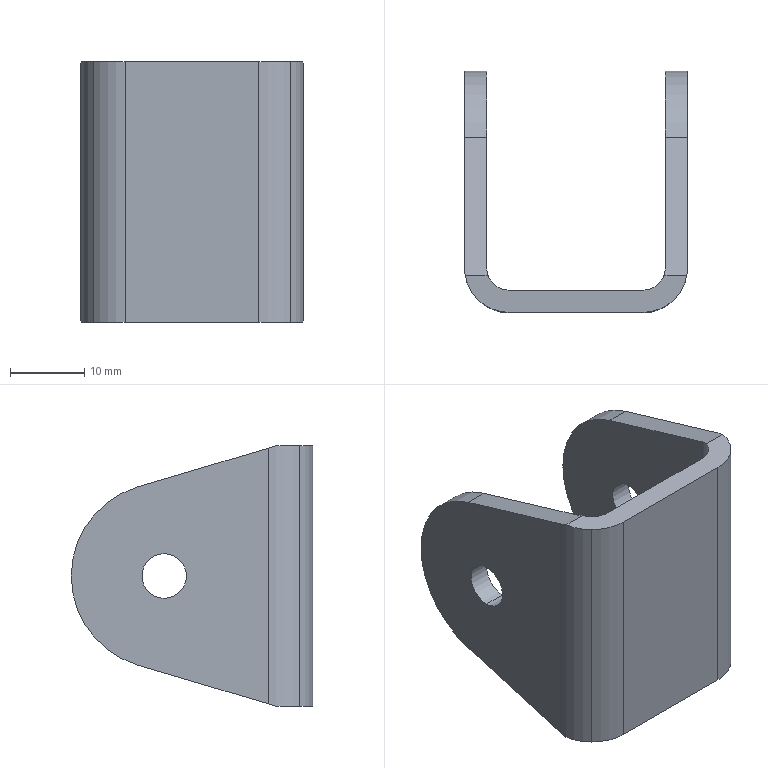Part | SolidWorks | features BaseBody 1 | 1 solid | 26 faces | box 30 x 32.5 x 35 mm | volume 7224 mm3 | cylinder 14 | plane 12 | commonest cylinder face diameters 6 x8 12 x4 25 x2
STEP:
#1=CARTESIAN_POINT('',(6.626,51.912,-683.821));
#2=VERTEX_POINT('',#1);
#3=CARTESIAN_POINT('',(6.626,51.912,-689.821));
#4=VERTEX_POINT('',#3);
#5=CARTESIAN_POINT('',(6.626,51.912,-686.821));
#6=DIRECTION('',(1.,0.,0.));
#7=DIRECTION('',(0.,0.,-1.));
#8=AXIS2_PLACEMENT_3D('',#5,#6,#7);
#9=CIRCLE('',#8,3.);
#10=EDGE_CURVE('',#2,#4,#9,.T.);
#11=ORIENTED_EDGE('',*,*,#10,.F.);
#12=CARTESIAN_POINT('',(9.626,51.912,-683.821));
#13=VERTEX_POINT('',#12);
#14=CARTESIAN_POINT('',(20.626,51.912,-683.821));
#15=DIRECTION('',(1.,0.,0.));
#16=VECTOR('',#15,1000.);
#17=LINE('',#14,#16);
#18=EDGE_CURVE('',#2,#13,#17,.T.);
#19=ORIENTED_EDGE('',*,*,#18,.T.);
#20=CARTESIAN_POINT('',(9.626,51.912,-689.821));
#21=VERTEX_POINT('',#20);
#22=CARTESIAN_POINT('',(9.626,51.912,-686.821));
#23=DIRECTION('',(-1.,0.,0.));
#24=DIRECTION('',(0.,0.,-1.));
#25=AXIS2_PLACEMENT_3D('',#22,#23,#24);
#26=CIRCLE('',#25,3.);
#27=EDGE_CURVE('',#21,#13,#26,.T.);
#28=ORIENTED_EDGE('',*,*,#27,.F.);
#29=CARTESIAN_POINT('',(20.626,51.912,-689.821));
#30=DIRECTION('',(1.,0.,0.));
#31=VECTOR('',#30,1000.);
#32=LINE('',#29,#31);
#33=EDGE_CURVE('',#4,#21,#32,.T.);
#34=ORIENTED_EDGE('',*,*,#33,.F.);
#35=EDGE_LOOP('',(#11,#19,#28,#34));
#36=FACE_OUTER_BOUND('',#35,.T.);
#37=CARTESIAN_POINT('',(20.626,51.912,-686.821));
#38=DIRECTION('',(1.,0.,0.));
#39=DIRECTION('',(0.,0.,-1.));
#40=AXIS2_PLACEMENT_3D('',#37,#38,#39);
#41=CYLINDRICAL_SURFACE('',#40,3.);
#42=ADVANCED_FACE('',(#36),#41,.F.);
#43=CARTESIAN_POINT('',(33.626,51.912,-683.821));
#44=VERTEX_POINT('',#43);
#45=CARTESIAN_POINT('',(33.626,51.912,-689.821));
#46=VERTEX_POINT('',#45);
#47=CARTESIAN_POINT('',(33.626,51.912,-686.821));
#48=DIRECTION('',(1.,0.,0.));
#49=DIRECTION('',(0.,0.,-1.));
#50=AXIS2_PLACEMENT_3D('',#47,#48,#49);
#51=CIRCLE('',#50,3.);
#52=EDGE_CURVE('',#44,#46,#51,.T.);
#53=ORIENTED_EDGE('',*,*,#52,.F.);
#54=CARTESIAN_POINT('',(36.626,51.912,-683.821));
#55=VERTEX_POINT('',#54);
#56=CARTESIAN_POINT('',(20.626,51.912,-683.821));
#57=DIRECTION('',(1.,0.,0.));
#58=VECTOR('',#57,1000.);
#59=LINE('',#56,#58);
#60=EDGE_CURVE('',#44,#55,#59,.T.);
#61=ORIENTED_EDGE('',*,*,#60,.T.);
#62=CARTESIAN_POINT('',(36.626,51.912,-689.821));
#63=VERTEX_POINT('',#62);
#64=CARTESIAN_POINT('',(36.626,51.912,-686.821));
#65=DIRECTION('',(-1.,0.,0.));
#66=DIRECTION('',(0.,0.,-1.));
#67=AXIS2_PLACEMENT_3D('',#64,#65,#66);
#68=CIRCLE('',#67,3.);
#69=EDGE_CURVE('',#63,#55,#68,.T.);
#70=ORIENTED_EDGE('',*,*,#69,.F.);
#71=CARTESIAN_POINT('',(20.626,51.912,-689.821));
#72=DIRECTION('',(1.,0.,0.));
#73=VECTOR('',#72,1000.);
#74=LINE('',#71,#73);
#75=EDGE_CURVE('',#46,#63,#74,.T.);
#76=ORIENTED_EDGE('',*,*,#75,.F.);
#77=EDGE_LOOP('',(#53,#61,#70,#76));
#78=FACE_OUTER_BOUND('',#77,.T.);
#79=CARTESIAN_POINT('',(20.626,51.912,-686.821));
#80=DIRECTION('',(1.,0.,0.));
#81=DIRECTION('',(0.,0.,-1.));
#82=AXIS2_PLACEMENT_3D('',#79,#80,#81);
#83=CYLINDRICAL_SURFACE('',#82,3.);
#84=ADVANCED_FACE('',(#78),#83,.F.);
#85=CARTESIAN_POINT('',(30.626,31.912,-704.321));
#86=VERTEX_POINT('',#85);
#87=CARTESIAN_POINT('',(34.868,33.67,-704.321));
#88=VERTEX_POINT('',#87);
#89=CARTESIAN_POINT('',(30.626,37.912,-704.321));
#90=DIRECTION('',(0.,0.,1.));
#91=DIRECTION('',(0.7071,-0.7071,0.));
#92=AXIS2_PLACEMENT_3D('',#89,#90,#91);
#93=CIRCLE('',#92,6.);
#94=EDGE_CURVE('',#86,#88,#93,.T.);
#95=ORIENTED_EDGE('',*,*,#94,.T.);
#96=CARTESIAN_POINT('',(34.868,33.67,-669.321));
#97=VERTEX_POINT('',#96);
#98=CARTESIAN_POINT('',(34.868,33.67,-695.571));
#99=DIRECTION('',(0.,0.,1.));
#100=VECTOR('',#99,1000.);
#101=LINE('',#98,#100);
#102=EDGE_CURVE('',#88,#97,#101,.T.);
#103=ORIENTED_EDGE('',*,*,#102,.T.);
#104=CARTESIAN_POINT('',(30.626,31.912,-669.321));
#105=VERTEX_POINT('',#104);
#106=CARTESIAN_POINT('',(30.626,37.912,-669.321));
#107=DIRECTION('',(0.,0.,-1.));
#108=DIRECTION('',(0.7071,-0.7071,0.));
#109=AXIS2_PLACEMENT_3D('',#106,#107,#108);
#110=CIRCLE('',#109,6.);
#111=EDGE_CURVE('',#97,#105,#110,.T.);
#112=ORIENTED_EDGE('',*,*,#111,.T.);
#113=CARTESIAN_POINT('',(30.626,31.912,-695.571));
#114=DIRECTION('',(0.,0.,-1.));
#115=VECTOR('',#114,1000.);
#116=LINE('',#113,#115);
#117=EDGE_CURVE('',#105,#86,#116,.T.);
#118=ORIENTED_EDGE('',*,*,#117,.T.);
#119=EDGE_LOOP('',(#95,#103,#112,#118));
#120=FACE_OUTER_BOUND('',#119,.T.);
#121=CARTESIAN_POINT('',(30.626,37.912,-695.571));
#122=DIRECTION('',(0.,0.,1.));
#123=DIRECTION('',(0.7071,-0.7071,0.));
#124=AXIS2_PLACEMENT_3D('',#121,#122,#123);
#125=CYLINDRICAL_SURFACE('',#124,6.);
#126=ADVANCED_FACE('',(#120),#125,.T.);
#127=CARTESIAN_POINT('',(6.71,36.912,-704.321));
#128=VERTEX_POINT('',#127);
#129=CARTESIAN_POINT('',(8.383,33.67,-704.321));
#130=VERTEX_POINT('',#129);
#131=CARTESIAN_POINT('',(12.626,37.912,-704.321));
#132=DIRECTION('',(0.,0.,1.));
#133=DIRECTION('',(-0.7071,-0.7071,0.));
#134=AXIS2_PLACEMENT_3D('',#131,#132,#133);
#135=CIRCLE('',#134,6.);
#136=EDGE_CURVE('',#128,#130,#135,.T.);
#137=ORIENTED_EDGE('',*,*,#136,.T.);
#138=CARTESIAN_POINT('',(8.383,33.67,-669.321));
#139=VERTEX_POINT('',#138);
#140=CARTESIAN_POINT('',(8.383,33.67,-695.571));
#141=DIRECTION('',(0.,0.,1.));
#142=VECTOR('',#141,1000.);
#143=LINE('',#140,#142);
#144=EDGE_CURVE('',#130,#139,#143,.T.);
#145=ORIENTED_EDGE('',*,*,#144,.T.);
#146=CARTESIAN_POINT('',(6.71,36.912,-669.321));
#147=VERTEX_POINT('',#146);
#148=CARTESIAN_POINT('',(12.626,37.912,-669.321));
#149=DIRECTION('',(0.,0.,-1.));
#150=DIRECTION('',(-0.7071,-0.7071,0.));
#151=AXIS2_PLACEMENT_3D('',#148,#149,#150);
#152=CIRCLE('',#151,6.);
#153=EDGE_CURVE('',#139,#147,#152,.T.);
#154=ORIENTED_EDGE('',*,*,#153,.T.);
#155=CARTESIAN_POINT('',(6.626,37.912,-669.619));
#156=VERTEX_POINT('',#155);
#157=CARTESIAN_POINT('',(6.71,36.912,-669.321));
#158=CARTESIAN_POINT('',(6.654,37.243,-669.42));
#159=CARTESIAN_POINT('',(6.626,37.577,-669.519));
#160=CARTESIAN_POINT('',(6.626,37.912,-669.619));
#161=(BOUNDED_CURVE()B_SPLINE_CURVE(3,(#157,#158,#159,#160),.UNSPECIFIED.,.F.,.T.)B_SPLINE_CURVE_WITH_KNOTS((4,4),(1.403,1.571),.UNSPECIFIED.)CURVE()GEOMETRIC_REPRESENTATION_ITEM()RATIONAL_B_SPLINE_CURVE((1.,0.9977,0.9977,1.))REPRESENTATION_ITEM(''));
#162=EDGE_CURVE('',#147,#156,#161,.T.);
#163=ORIENTED_EDGE('',*,*,#162,.T.);
#164=CARTESIAN_POINT('',(6.626,37.912,-704.024));
#165=VERTEX_POINT('',#164);
#166=CARTESIAN_POINT('',(6.626,37.912,-695.571));
#167=DIRECTION('',(0.,0.,-1.));
#168=VECTOR('',#167,1000.);
#169=LINE('',#166,#168);
#170=EDGE_CURVE('',#156,#165,#169,.T.);
#171=ORIENTED_EDGE('',*,*,#170,.T.);
#172=CARTESIAN_POINT('',(6.626,37.912,-704.024));
#173=CARTESIAN_POINT('',(6.626,37.577,-704.124));
#174=CARTESIAN_POINT('',(6.654,37.243,-704.223));
#175=CARTESIAN_POINT('',(6.71,36.912,-704.321));
#176=(BOUNDED_CURVE()B_SPLINE_CURVE(3,(#172,#173,#174,#175),.UNSPECIFIED.,.F.,.F.)B_SPLINE_CURVE_WITH_KNOTS((4,4),(4.712,4.88),.UNSPECIFIED.)CURVE()GEOMETRIC_REPRESENTATION_ITEM()RATIONAL_B_SPLINE_CURVE((1.,0.9977,0.9977,1.))REPRESENTATION_ITEM(''));
#177=EDGE_CURVE('',#165,#128,#176,.T.);
#178=ORIENTED_EDGE('',*,*,#177,.T.);
#179=EDGE_LOOP('',(#137,#145,#154,#163,#171,#178));
#180=FACE_OUTER_BOUND('',#179,.T.);
#181=CARTESIAN_POINT('',(12.626,37.912,-695.571));
#182=DIRECTION('',(0.,0.,1.));
#183=DIRECTION('',(-0.7071,-0.7071,0.));
#184=AXIS2_PLACEMENT_3D('',#181,#182,#183);
#185=CYLINDRICAL_SURFACE('',#184,6.);
#186=ADVANCED_FACE('',(#180),#185,.T.);
#187=CARTESIAN_POINT('',(30.626,34.912,-669.321));
#188=VERTEX_POINT('',#187);
#189=CARTESIAN_POINT('',(32.747,35.791,-669.321));
#190=VERTEX_POINT('',#189);
#191=CARTESIAN_POINT('',(30.626,37.912,-669.321));
#192=DIRECTION('',(0.,0.,1.));
#193=DIRECTION('',(0.7071,-0.7071,0.));
#194=AXIS2_PLACEMENT_3D('',#191,#192,#193);
#195=CIRCLE('',#194,3.);
#196=EDGE_CURVE('',#188,#190,#195,.T.);
#197=ORIENTED_EDGE('',*,*,#196,.T.);
#198=CARTESIAN_POINT('',(32.747,35.791,-704.321));
#199=VERTEX_POINT('',#198);
#200=CARTESIAN_POINT('',(32.747,35.791,-669.321));
#201=DIRECTION('',(0.,0.,-1.));
#202=VECTOR('',#201,1000.);
#203=LINE('',#200,#202);
#204=EDGE_CURVE('',#190,#199,#203,.T.);
#205=ORIENTED_EDGE('',*,*,#204,.T.);
#206=CARTESIAN_POINT('',(30.626,34.912,-704.321));
#207=VERTEX_POINT('',#206);
#208=CARTESIAN_POINT('',(30.626,37.912,-704.321));
#209=DIRECTION('',(0.,0.,1.));
#210=DIRECTION('',(0.7071,-0.7071,0.));
#211=AXIS2_PLACEMENT_3D('',#208,#209,#210);
#212=CIRCLE('',#211,3.);
#213=EDGE_CURVE('',#207,#199,#212,.T.);
#214=ORIENTED_EDGE('',*,*,#213,.F.);
#215=CARTESIAN_POINT('',(30.626,34.912,-669.321));
#216=DIRECTION('',(0.,0.,1.));
#217=VECTOR('',#216,1000.);
#218=LINE('',#215,#217);
#219=EDGE_CURVE('',#207,#188,#218,.T.);
#220=ORIENTED_EDGE('',*,*,#219,.T.);
#221=EDGE_LOOP('',(#197,#205,#214,#220));
#222=FACE_OUTER_BOUND('',#221,.T.);
#223=CARTESIAN_POINT('',(30.626,37.912,-669.321));
#224=DIRECTION('',(0.,0.,-1.));
#225=DIRECTION('',(0.7071,-0.7071,0.));
#226=AXIS2_PLACEMENT_3D('',#223,#224,#225);
#227=CYLINDRICAL_SURFACE('',#226,3.);
#228=ADVANCED_FACE('',(#222),#227,.F.);
#229=CARTESIAN_POINT('',(10.504,35.791,-669.321));
#230=VERTEX_POINT('',#229);
#231=CARTESIAN_POINT('',(9.797,36.912,-669.321));
#232=VERTEX_POINT('',#231);
#233=CARTESIAN_POINT('',(12.626,37.912,-669.321));
#234=DIRECTION('',(0.,0.,-1.));
#235=DIRECTION('',(-0.7071,-0.7071,0.));
#236=AXIS2_PLACEMENT_3D('',#233,#234,#235);
#237=CIRCLE('',#236,3.);
#238=EDGE_CURVE('',#230,#232,#237,.T.);
#239=ORIENTED_EDGE('',*,*,#238,.F.);
#240=CARTESIAN_POINT('',(10.504,35.791,-704.321));
#241=VERTEX_POINT('',#240);
#242=CARTESIAN_POINT('',(10.504,35.791,-669.321));
#243=DIRECTION('',(0.,0.,-1.));
#244=VECTOR('',#243,1000.);
#245=LINE('',#242,#244);
#246=EDGE_CURVE('',#230,#241,#245,.T.);
#247=ORIENTED_EDGE('',*,*,#246,.T.);
#248=CARTESIAN_POINT('',(9.797,36.912,-704.321));
#249=VERTEX_POINT('',#248);
#250=CARTESIAN_POINT('',(12.626,37.912,-704.321));
#251=DIRECTION('',(0.,0.,-1.));
#252=DIRECTION('',(-0.7071,-0.7071,0.));
#253=AXIS2_PLACEMENT_3D('',#250,#251,#252);
#254=CIRCLE('',#253,3.);
#255=EDGE_CURVE('',#241,#249,#254,.T.);
#256=ORIENTED_EDGE('',*,*,#255,.T.);
#257=CARTESIAN_POINT('',(9.626,37.912,-704.024));
#258=VERTEX_POINT('',#257);
#259=CARTESIAN_POINT('',(9.626,37.912,-704.024));
#260=CARTESIAN_POINT('',(9.626,37.571,-704.126));
#261=CARTESIAN_POINT('',(9.683,37.234,-704.226));
#262=CARTESIAN_POINT('',(9.797,36.912,-704.321));
#263=(BOUNDED_CURVE()B_SPLINE_CURVE(3,(#259,#260,#261,#262),.UNSPECIFIED.,.F.,.F.)B_SPLINE_CURVE_WITH_KNOTS((4,4),(4.712,5.052),.UNSPECIFIED.)CURVE()GEOMETRIC_REPRESENTATION_ITEM()RATIONAL_B_SPLINE_CURVE((1.,0.9904,0.9904,1.))REPRESENTATION_ITEM(''));
#264=EDGE_CURVE('',#258,#249,#263,.T.);
#265=ORIENTED_EDGE('',*,*,#264,.F.);
#266=CARTESIAN_POINT('',(9.626,37.912,-669.619));
#267=VERTEX_POINT('',#266);
#268=CARTESIAN_POINT('',(9.626,37.912,-669.321));
#269=DIRECTION('',(0.,0.,1.));
#270=VECTOR('',#269,1000.);
#271=LINE('',#268,#270);
#272=EDGE_CURVE('',#258,#267,#271,.T.);
#273=ORIENTED_EDGE('',*,*,#272,.T.);
#274=CARTESIAN_POINT('',(9.626,37.912,-669.619));
#275=CARTESIAN_POINT('',(9.626,37.571,-669.517));
#276=CARTESIAN_POINT('',(9.683,37.234,-669.417));
#277=CARTESIAN_POINT('',(9.797,36.912,-669.321));
#278=(BOUNDED_CURVE()B_SPLINE_CURVE(3,(#274,#275,#276,#277),.UNSPECIFIED.,.F.,.F.)B_SPLINE_CURVE_WITH_KNOTS((4,4),(4.712,5.052),.UNSPECIFIED.)CURVE()GEOMETRIC_REPRESENTATION_ITEM()RATIONAL_B_SPLINE_CURVE((1.,0.9904,0.9904,1.))REPRESENTATION_ITEM(''));
#279=EDGE_CURVE('',#267,#232,#278,.T.);
#280=ORIENTED_EDGE('',*,*,#279,.T.);
#281=EDGE_LOOP('',(#239,#247,#256,#265,#273,#280));
#282=FACE_OUTER_BOUND('',#281,.T.);
#283=CARTESIAN_POINT('',(12.626,37.912,-669.321));
#284=DIRECTION('',(0.,0.,-1.));
#285=DIRECTION('',(-0.7071,-0.7071,0.));
#286=AXIS2_PLACEMENT_3D('',#283,#284,#285);
#287=CYLINDRICAL_SURFACE('',#286,3.);
#288=ADVANCED_FACE('',(#282),#287,.F.);
#289=ORIENTED_EDGE('',*,*,#69,.T.);
#290=CARTESIAN_POINT('',(36.626,51.912,-686.821));
#291=DIRECTION('',(-1.,0.,0.));
#292=DIRECTION('',(0.,0.,-1.));
#293=AXIS2_PLACEMENT_3D('',#290,#291,#292);
#294=CIRCLE('',#293,3.);
#295=EDGE_CURVE('',#55,#63,#294,.T.);
#296=ORIENTED_EDGE('',*,*,#295,.T.);
#297=EDGE_LOOP('',(#289,#296));
#298=FACE_BOUND('',#297,.T.);
#299=CARTESIAN_POINT('',(36.626,37.912,-704.024));
#300=VERTEX_POINT('',#299);
#301=CARTESIAN_POINT('',(36.626,37.912,-669.619));
#302=VERTEX_POINT('',#301);
#303=CARTESIAN_POINT('',(36.626,37.912,-695.571));
#304=DIRECTION('',(0.,0.,1.));
#305=VECTOR('',#304,1000.);
#306=LINE('',#303,#305);
#307=EDGE_CURVE('',#300,#302,#306,.T.);
#308=ORIENTED_EDGE('',*,*,#307,.F.);
#309=CARTESIAN_POINT('',(36.626,55.474,-698.803));
#310=VERTEX_POINT('',#309);
#311=CARTESIAN_POINT('',(36.626,55.474,-698.803));
#312=DIRECTION('',(0.,-0.9585,-0.285));
#313=VECTOR('',#312,1000.);
#314=LINE('',#311,#313);
#315=EDGE_CURVE('',#310,#300,#314,.T.);
#316=ORIENTED_EDGE('',*,*,#315,.F.);
#317=CARTESIAN_POINT('',(36.626,55.474,-674.84));
#318=VERTEX_POINT('',#317);
#319=CARTESIAN_POINT('',(36.626,51.912,-686.821));
#320=DIRECTION('',(-1.,0.,0.));
#321=DIRECTION('',(0.,0.285,0.9585));
#322=AXIS2_PLACEMENT_3D('',#319,#320,#321);
#323=CIRCLE('',#322,12.5);
#324=EDGE_CURVE('',#318,#310,#323,.T.);
#325=ORIENTED_EDGE('',*,*,#324,.F.);
#326=CARTESIAN_POINT('',(36.626,36.912,-669.321));
#327=DIRECTION('',(0.,0.9585,-0.285));
#328=VECTOR('',#327,1000.);
#329=LINE('',#326,#328);
#330=EDGE_CURVE('',#302,#318,#329,.T.);
#331=ORIENTED_EDGE('',*,*,#330,.F.);
#332=EDGE_LOOP('',(#308,#316,#325,#331));
#333=FACE_OUTER_BOUND('',#332,.T.);
#334=CARTESIAN_POINT('',(36.626,43.822,-686.821));
#335=DIRECTION('',(-1.,0.,0.));
#336=DIRECTION('',(0.,0.,1.));
#337=AXIS2_PLACEMENT_3D('',#334,#335,#336);
#338=PLANE('',#337);
#339=ADVANCED_FACE('',(#298,#333),#338,.F.);
#340=CARTESIAN_POINT('',(6.626,51.912,-686.821));
#341=DIRECTION('',(1.,0.,0.));
#342=DIRECTION('',(0.,0.,-1.));
#343=AXIS2_PLACEMENT_3D('',#340,#341,#342);
#344=CIRCLE('',#343,3.);
#345=EDGE_CURVE('',#4,#2,#344,.T.);
#346=ORIENTED_EDGE('',*,*,#345,.T.);
#347=ORIENTED_EDGE('',*,*,#10,.T.);
#348=EDGE_LOOP('',(#346,#347));
#349=FACE_BOUND('',#348,.T.);
#350=ORIENTED_EDGE('',*,*,#170,.F.);
#351=CARTESIAN_POINT('',(6.626,55.474,-674.84));
#352=VERTEX_POINT('',#351);
#353=CARTESIAN_POINT('',(6.626,36.912,-669.321));
#354=DIRECTION('',(0.,0.9585,-0.285));
#355=VECTOR('',#354,1000.);
#356=LINE('',#353,#355);
#357=EDGE_CURVE('',#156,#352,#356,.T.);
#358=ORIENTED_EDGE('',*,*,#357,.T.);
#359=CARTESIAN_POINT('',(6.626,55.474,-698.803));
#360=VERTEX_POINT('',#359);
#361=CARTESIAN_POINT('',(6.626,51.912,-686.821));
#362=DIRECTION('',(-1.,0.,0.));
#363=DIRECTION('',(0.,0.285,0.9585));
#364=AXIS2_PLACEMENT_3D('',#361,#362,#363);
#365=CIRCLE('',#364,12.5);
#366=EDGE_CURVE('',#352,#360,#365,.T.);
#367=ORIENTED_EDGE('',*,*,#366,.T.);
#368=CARTESIAN_POINT('',(6.626,55.474,-698.803));
#369=DIRECTION('',(0.,-0.9585,-0.285));
#370=VECTOR('',#369,1000.);
#371=LINE('',#368,#370);
#372=EDGE_CURVE('',#360,#165,#371,.T.);
#373=ORIENTED_EDGE('',*,*,#372,.T.);
#374=EDGE_LOOP('',(#350,#358,#367,#373));
#375=FACE_OUTER_BOUND('',#374,.T.);
#376=CARTESIAN_POINT('',(6.626,43.822,-686.821));
#377=DIRECTION('',(-1.,0.,0.));
#378=DIRECTION('',(0.,0.,1.));
#379=AXIS2_PLACEMENT_3D('',#376,#377,#378);
#380=PLANE('',#379);
#381=ADVANCED_FACE('',(#349,#375),#380,.T.);
#382=CARTESIAN_POINT('',(33.626,55.474,-698.803));
#383=VERTEX_POINT('',#382);
#384=CARTESIAN_POINT('',(33.626,55.474,-674.84));
#385=VERTEX_POINT('',#384);
#386=CARTESIAN_POINT('',(33.626,51.912,-686.821));
#387=DIRECTION('',(1.,0.,0.));
#388=DIRECTION('',(0.,0.285,0.9585));
#389=AXIS2_PLACEMENT_3D('',#386,#387,#388);
#390=CIRCLE('',#389,12.5);
#391=EDGE_CURVE('',#383,#385,#390,.T.);
#392=ORIENTED_EDGE('',*,*,#391,.T.);
#393=CARTESIAN_POINT('',(36.626,55.474,-674.84));
#394=DIRECTION('',(-1.,0.,0.));
#395=VECTOR('',#394,1000.);
#396=LINE('',#393,#395);
#397=EDGE_CURVE('',#318,#385,#396,.T.);
#398=ORIENTED_EDGE('',*,*,#397,.F.);
#399=ORIENTED_EDGE('',*,*,#324,.T.);
#400=CARTESIAN_POINT('',(36.626,55.474,-698.803));
#401=DIRECTION('',(-1.,0.,0.));
#402=VECTOR('',#401,1000.);
#403=LINE('',#400,#402);
#404=EDGE_CURVE('',#310,#383,#403,.T.);
#405=ORIENTED_EDGE('',*,*,#404,.T.);
#406=EDGE_LOOP('',(#392,#398,#399,#405));
#407=FACE_OUTER_BOUND('',#406,.T.);
#408=CARTESIAN_POINT('',(36.626,51.912,-686.821));
#409=DIRECTION('',(-1.,0.,0.));
#410=DIRECTION('',(0.,0.285,0.9585));
#411=AXIS2_PLACEMENT_3D('',#408,#409,#410);
#412=CYLINDRICAL_SURFACE('',#411,12.5);
#413=ADVANCED_FACE('',(#407),#412,.T.);
#414=CARTESIAN_POINT('',(9.626,55.474,-674.84));
#415=VERTEX_POINT('',#414);
#416=CARTESIAN_POINT('',(9.626,55.474,-698.803));
#417=VERTEX_POINT('',#416);
#418=CARTESIAN_POINT('',(9.626,51.912,-686.821));
#419=DIRECTION('',(-1.,0.,0.));
#420=DIRECTION('',(0.,0.285,0.9585));
#421=AXIS2_PLACEMENT_3D('',#418,#419,#420);
#422=CIRCLE('',#421,12.5);
#423=EDGE_CURVE('',#415,#417,#422,.T.);
#424=ORIENTED_EDGE('',*,*,#423,.T.);
#425=CARTESIAN_POINT('',(36.626,55.474,-698.803));
#426=DIRECTION('',(-1.,0.,0.));
#427=VECTOR('',#426,1000.);
#428=LINE('',#425,#427);
#429=EDGE_CURVE('',#417,#360,#428,.T.);
#430=ORIENTED_EDGE('',*,*,#429,.T.);
#431=ORIENTED_EDGE('',*,*,#366,.F.);
#432=CARTESIAN_POINT('',(36.626,55.474,-674.84));
#433=DIRECTION('',(-1.,0.,0.));
#434=VECTOR('',#433,1000.);
#435=LINE('',#432,#434);
#436=EDGE_CURVE('',#415,#352,#435,.T.);
#437=ORIENTED_EDGE('',*,*,#436,.F.);
#438=EDGE_LOOP('',(#424,#430,#431,#437));
#439=FACE_OUTER_BOUND('',#438,.T.);
#440=CARTESIAN_POINT('',(36.626,51.912,-686.821));
#441=DIRECTION('',(-1.,0.,0.));
#442=DIRECTION('',(0.,0.285,0.9585));
#443=AXIS2_PLACEMENT_3D('',#440,#441,#442);
#444=CYLINDRICAL_SURFACE('',#443,12.5);
#445=ADVANCED_FACE('',(#439),#444,.T.);
#446=CARTESIAN_POINT('',(36.542,36.912,-669.321));
#447=VERTEX_POINT('',#446);
#448=CARTESIAN_POINT('',(36.626,37.912,-669.619));
#449=CARTESIAN_POINT('',(36.626,37.577,-669.519));
#450=CARTESIAN_POINT('',(36.598,37.243,-669.42));
#451=CARTESIAN_POINT('',(36.542,36.912,-669.321));
#452=(BOUNDED_CURVE()B_SPLINE_CURVE(3,(#448,#449,#450,#451),.UNSPECIFIED.,.F.,.F.)B_SPLINE_CURVE_WITH_KNOTS((4,4),(4.712,4.88),.UNSPECIFIED.)CURVE()GEOMETRIC_REPRESENTATION_ITEM()RATIONAL_B_SPLINE_CURVE((1.,0.9977,0.9977,1.))REPRESENTATION_ITEM(''));
#453=EDGE_CURVE('',#302,#447,#452,.T.);
#454=ORIENTED_EDGE('',*,*,#453,.F.);
#455=ORIENTED_EDGE('',*,*,#330,.T.);
#456=ORIENTED_EDGE('',*,*,#397,.T.);
#457=CARTESIAN_POINT('',(33.626,37.912,-669.619));
#458=VERTEX_POINT('',#457);
#459=CARTESIAN_POINT('',(33.626,51.202,-673.569));
#460=DIRECTION('',(0.,-0.9585,0.285));
#461=VECTOR('',#460,1000.);
#462=LINE('',#459,#461);
#463=EDGE_CURVE('',#385,#458,#462,.T.);
#464=ORIENTED_EDGE('',*,*,#463,.T.);
#465=CARTESIAN_POINT('',(33.454,36.912,-669.321));
#466=VERTEX_POINT('',#465);
#467=CARTESIAN_POINT('',(33.626,37.912,-669.619));
#468=CARTESIAN_POINT('',(33.626,37.571,-669.517));
#469=CARTESIAN_POINT('',(33.568,37.234,-669.417));
#470=CARTESIAN_POINT('',(33.454,36.912,-669.321));
#471=(BOUNDED_CURVE()B_SPLINE_CURVE(3,(#467,#468,#469,#470),.UNSPECIFIED.,.F.,.F.)B_SPLINE_CURVE_WITH_KNOTS((4,4),(4.712,5.052),.UNSPECIFIED.)CURVE()GEOMETRIC_REPRESENTATION_ITEM()RATIONAL_B_SPLINE_CURVE((1.,0.9904,0.9904,1.))REPRESENTATION_ITEM(''));
#472=EDGE_CURVE('',#458,#466,#471,.T.);
#473=ORIENTED_EDGE('',*,*,#472,.T.);
#474=CARTESIAN_POINT('',(36.626,36.912,-669.321));
#475=DIRECTION('',(-1.,0.,0.));
#476=VECTOR('',#475,1000.);
#477=LINE('',#474,#476);
#478=EDGE_CURVE('',#447,#466,#477,.T.);
#479=ORIENTED_EDGE('',*,*,#478,.F.);
#480=EDGE_LOOP('',(#454,#455,#456,#464,#473,#479));
#481=FACE_OUTER_BOUND('',#480,.T.);
#482=CARTESIAN_POINT('',(36.626,36.912,-669.321));
#483=DIRECTION('',(0.,0.285,0.9585));
#484=DIRECTION('',(1.,0.,0.));
#485=AXIS2_PLACEMENT_3D('',#482,#483,#484);
#486=PLANE('',#485);
#487=ADVANCED_FACE('',(#481),#486,.T.);
#488=ORIENTED_EDGE('',*,*,#162,.F.);
#489=CARTESIAN_POINT('',(36.626,36.912,-669.321));
#490=DIRECTION('',(-1.,0.,0.));
#491=VECTOR('',#490,1000.);
#492=LINE('',#489,#491);
#493=EDGE_CURVE('',#232,#147,#492,.T.);
#494=ORIENTED_EDGE('',*,*,#493,.F.);
#495=ORIENTED_EDGE('',*,*,#279,.F.);
#496=CARTESIAN_POINT('',(9.626,35.994,-669.048));
#497=DIRECTION('',(0.,0.9585,-0.285));
#498=VECTOR('',#497,1000.);
#499=LINE('',#496,#498);
#500=EDGE_CURVE('',#267,#415,#499,.T.);
#501=ORIENTED_EDGE('',*,*,#500,.T.);
#502=ORIENTED_EDGE('',*,*,#436,.T.);
#503=ORIENTED_EDGE('',*,*,#357,.F.);
#504=EDGE_LOOP('',(#488,#494,#495,#501,#502,#503));
#505=FACE_OUTER_BOUND('',#504,.T.);
#506=CARTESIAN_POINT('',(36.626,36.912,-669.321));
#507=DIRECTION('',(0.,0.285,0.9585));
#508=DIRECTION('',(1.,0.,0.));
#509=AXIS2_PLACEMENT_3D('',#506,#507,#508);
#510=PLANE('',#509);
#511=ADVANCED_FACE('',(#505),#510,.T.);
#512=CARTESIAN_POINT('',(30.626,37.912,-669.321));
#513=DIRECTION('',(0.,0.,-1.));
#514=DIRECTION('',(0.7071,-0.7071,0.));
#515=AXIS2_PLACEMENT_3D('',#512,#513,#514);
#516=CIRCLE('',#515,6.);
#517=EDGE_CURVE('',#447,#97,#516,.T.);
#518=ORIENTED_EDGE('',*,*,#517,.F.);
#519=ORIENTED_EDGE('',*,*,#478,.T.);
#520=CARTESIAN_POINT('',(30.626,37.912,-669.321));
#521=DIRECTION('',(0.,0.,1.));
#522=DIRECTION('',(0.7071,-0.7071,0.));
#523=AXIS2_PLACEMENT_3D('',#520,#521,#522);
#524=CIRCLE('',#523,3.);
#525=EDGE_CURVE('',#190,#466,#524,.T.);
#526=ORIENTED_EDGE('',*,*,#525,.F.);
#527=ORIENTED_EDGE('',*,*,#196,.F.);
#528=CARTESIAN_POINT('',(12.626,34.912,-669.321));
#529=VERTEX_POINT('',#528);
#530=CARTESIAN_POINT('',(35.126,34.912,-669.321));
#531=DIRECTION('',(-1.,0.,0.));
#532=VECTOR('',#531,1000.);
#533=LINE('',#530,#532);
#534=EDGE_CURVE('',#188,#529,#533,.T.);
#535=ORIENTED_EDGE('',*,*,#534,.T.);
#536=CARTESIAN_POINT('',(12.626,37.912,-669.321));
#537=DIRECTION('',(0.,0.,-1.));
#538=DIRECTION('',(-0.7071,-0.7071,0.));
#539=AXIS2_PLACEMENT_3D('',#536,#537,#538);
#540=CIRCLE('',#539,3.);
#541=EDGE_CURVE('',#529,#230,#540,.T.);
#542=ORIENTED_EDGE('',*,*,#541,.T.);
#543=ORIENTED_EDGE('',*,*,#238,.T.);
#544=ORIENTED_EDGE('',*,*,#493,.T.);
#545=ORIENTED_EDGE('',*,*,#153,.F.);
#546=CARTESIAN_POINT('',(12.626,31.912,-669.321));
#547=VERTEX_POINT('',#546);
#548=CARTESIAN_POINT('',(12.626,37.912,-669.321));
#549=DIRECTION('',(0.,0.,-1.));
#550=DIRECTION('',(-0.7071,-0.7071,0.));
#551=AXIS2_PLACEMENT_3D('',#548,#549,#550);
#552=CIRCLE('',#551,6.);
#553=EDGE_CURVE('',#547,#139,#552,.T.);
#554=ORIENTED_EDGE('',*,*,#553,.F.);
#555=CARTESIAN_POINT('',(36.626,31.912,-669.321));
#556=DIRECTION('',(-1.,0.,0.));
#557=VECTOR('',#556,1000.);
#558=LINE('',#555,#557);
#559=EDGE_CURVE('',#105,#547,#558,.T.);
#560=ORIENTED_EDGE('',*,*,#559,.F.);
#561=ORIENTED_EDGE('',*,*,#111,.F.);
#562=EDGE_LOOP('',(#518,#519,#526,#527,#535,#542,#543,#544,#545,#554,#560,#561));
#563=FACE_OUTER_BOUND('',#562,.T.);
#564=CARTESIAN_POINT('',(36.626,31.912,-669.321));
#565=DIRECTION('',(0.,0.,1.));
#566=DIRECTION('',(0.,1.,0.));
#567=AXIS2_PLACEMENT_3D('',#564,#565,#566);
#568=PLANE('',#567);
#569=ADVANCED_FACE('',(#563),#568,.T.);
#570=ORIENTED_EDGE('',*,*,#27,.T.);
#571=CARTESIAN_POINT('',(9.626,51.912,-686.821));
#572=DIRECTION('',(-1.,0.,0.));
#573=DIRECTION('',(0.,0.,-1.));
#574=AXIS2_PLACEMENT_3D('',#571,#572,#573);
#575=CIRCLE('',#574,3.);
#576=EDGE_CURVE('',#13,#21,#575,.T.);
#577=ORIENTED_EDGE('',*,*,#576,.T.);
#578=EDGE_LOOP('',(#570,#577));
#579=FACE_BOUND('',#578,.T.);
#580=ORIENTED_EDGE('',*,*,#272,.F.);
#581=CARTESIAN_POINT('',(9.626,50.055,-700.414));
#582=DIRECTION('',(0.,-0.9585,-0.285));
#583=VECTOR('',#582,1000.);
#584=LINE('',#581,#583);
#585=EDGE_CURVE('',#417,#258,#584,.T.);
#586=ORIENTED_EDGE('',*,*,#585,.F.);
#587=ORIENTED_EDGE('',*,*,#423,.F.);
#588=ORIENTED_EDGE('',*,*,#500,.F.);
#589=EDGE_LOOP('',(#580,#586,#587,#588));
#590=FACE_OUTER_BOUND('',#589,.T.);
#591=CARTESIAN_POINT('',(9.626,34.912,-669.321));
#592=DIRECTION('',(-1.,0.,0.));
#593=DIRECTION('',(0.,-1.,0.));
#594=AXIS2_PLACEMENT_3D('',#591,#592,#593);
#595=PLANE('',#594);
#596=ADVANCED_FACE('',(#579,#590),#595,.F.);
#597=ORIENTED_EDGE('',*,*,#219,.F.);
#598=CARTESIAN_POINT('',(12.626,34.912,-704.321));
#599=VERTEX_POINT('',#598);
#600=CARTESIAN_POINT('',(35.126,34.912,-704.321));
#601=DIRECTION('',(1.,0.,0.));
#602=VECTOR('',#601,1000.);
#603=LINE('',#600,#602);
#604=EDGE_CURVE('',#599,#207,#603,.T.);
#605=ORIENTED_EDGE('',*,*,#604,.F.);
#606=CARTESIAN_POINT('',(12.626,34.912,-669.321));
#607=DIRECTION('',(0.,0.,-1.));
#608=VECTOR('',#607,1000.);
#609=LINE('',#606,#608);
#610=EDGE_CURVE('',#529,#599,#609,.T.);
#611=ORIENTED_EDGE('',*,*,#610,.F.);
#612=ORIENTED_EDGE('',*,*,#534,.F.);
#613=EDGE_LOOP('',(#597,#605,#611,#612));
#614=FACE_OUTER_BOUND('',#613,.T.);
#615=CARTESIAN_POINT('',(33.626,34.912,-669.321));
#616=DIRECTION('',(0.,-1.,0.));
#617=DIRECTION('',(1.,0.,0.));
#618=AXIS2_PLACEMENT_3D('',#615,#616,#617);
#619=PLANE('',#618);
#620=ADVANCED_FACE('',(#614),#619,.F.);
#621=ORIENTED_EDGE('',*,*,#246,.F.);
#622=ORIENTED_EDGE('',*,*,#541,.F.);
#623=ORIENTED_EDGE('',*,*,#610,.T.);
#624=CARTESIAN_POINT('',(12.626,37.912,-704.321));
#625=DIRECTION('',(0.,0.,-1.));
#626=DIRECTION('',(-0.7071,-0.7071,0.));
#627=AXIS2_PLACEMENT_3D('',#624,#625,#626);
#628=CIRCLE('',#627,3.);
#629=EDGE_CURVE('',#599,#241,#628,.T.);
#630=ORIENTED_EDGE('',*,*,#629,.T.);
#631=EDGE_LOOP('',(#621,#622,#623,#630));
#632=FACE_OUTER_BOUND('',#631,.T.);
#633=CARTESIAN_POINT('',(12.626,37.912,-669.321));
#634=DIRECTION('',(0.,0.,-1.));
#635=DIRECTION('',(-0.7071,-0.7071,0.));
#636=AXIS2_PLACEMENT_3D('',#633,#634,#635);
#637=CYLINDRICAL_SURFACE('',#636,3.);
#638=ADVANCED_FACE('',(#632),#637,.F.);
#639=CARTESIAN_POINT('',(33.626,51.912,-686.821));
#640=DIRECTION('',(1.,0.,0.));
#641=DIRECTION('',(0.,0.,-1.));
#642=AXIS2_PLACEMENT_3D('',#639,#640,#641);
#643=CIRCLE('',#642,3.);
#644=EDGE_CURVE('',#46,#44,#643,.T.);
#645=ORIENTED_EDGE('',*,*,#644,.T.);
#646=ORIENTED_EDGE('',*,*,#52,.T.);
#647=EDGE_LOOP('',(#645,#646));
#648=FACE_BOUND('',#647,.T.);
#649=CARTESIAN_POINT('',(33.626,37.912,-704.024));
#650=VERTEX_POINT('',#649);
#651=CARTESIAN_POINT('',(33.626,37.912,-669.321));
#652=DIRECTION('',(0.,0.,-1.));
#653=VECTOR('',#652,1000.);
#654=LINE('',#651,#653);
#655=EDGE_CURVE('',#458,#650,#654,.T.);
#656=ORIENTED_EDGE('',*,*,#655,.F.);
#657=ORIENTED_EDGE('',*,*,#463,.F.);
#658=ORIENTED_EDGE('',*,*,#391,.F.);
#659=CARTESIAN_POINT('',(33.626,65.263,-695.893));
#660=DIRECTION('',(0.,0.9585,0.285));
#661=VECTOR('',#660,1000.);
#662=LINE('',#659,#661);
#663=EDGE_CURVE('',#650,#383,#662,.T.);
#664=ORIENTED_EDGE('',*,*,#663,.F.);
#665=EDGE_LOOP('',(#656,#657,#658,#664));
#666=FACE_OUTER_BOUND('',#665,.T.);
#667=CARTESIAN_POINT('',(33.626,68.017,-669.321));
#668=DIRECTION('',(1.,0.,0.));
#669=DIRECTION('',(0.,-1.,0.));
#670=AXIS2_PLACEMENT_3D('',#667,#668,#669);
#671=PLANE('',#670);
#672=ADVANCED_FACE('',(#648,#666),#671,.F.);
#673=ORIENTED_EDGE('',*,*,#204,.F.);
#674=ORIENTED_EDGE('',*,*,#525,.T.);
#675=ORIENTED_EDGE('',*,*,#472,.F.);
#676=ORIENTED_EDGE('',*,*,#655,.T.);
#677=CARTESIAN_POINT('',(33.454,36.912,-704.321));
#678=VERTEX_POINT('',#677);
#679=CARTESIAN_POINT('',(33.626,37.912,-704.024));
#680=CARTESIAN_POINT('',(33.626,37.571,-704.126));
#681=CARTESIAN_POINT('',(33.568,37.234,-704.226));
#682=CARTESIAN_POINT('',(33.454,36.912,-704.321));
#683=(BOUNDED_CURVE()B_SPLINE_CURVE(3,(#679,#680,#681,#682),.UNSPECIFIED.,.F.,.F.)B_SPLINE_CURVE_WITH_KNOTS((4,4),(4.712,5.052),.UNSPECIFIED.)CURVE()GEOMETRIC_REPRESENTATION_ITEM()RATIONAL_B_SPLINE_CURVE((1.,0.9904,0.9904,1.))REPRESENTATION_ITEM(''));
#684=EDGE_CURVE('',#650,#678,#683,.T.);
#685=ORIENTED_EDGE('',*,*,#684,.T.);
#686=CARTESIAN_POINT('',(30.626,37.912,-704.321));
#687=DIRECTION('',(0.,0.,1.));
#688=DIRECTION('',(0.7071,-0.7071,0.));
#689=AXIS2_PLACEMENT_3D('',#686,#687,#688);
#690=CIRCLE('',#689,3.);
#691=EDGE_CURVE('',#199,#678,#690,.T.);
#692=ORIENTED_EDGE('',*,*,#691,.F.);
#693=EDGE_LOOP('',(#673,#674,#675,#676,#685,#692));
#694=FACE_OUTER_BOUND('',#693,.T.);
#695=CARTESIAN_POINT('',(30.626,37.912,-669.321));
#696=DIRECTION('',(0.,0.,-1.));
#697=DIRECTION('',(0.7071,-0.7071,0.));
#698=AXIS2_PLACEMENT_3D('',#695,#696,#697);
#699=CYLINDRICAL_SURFACE('',#698,3.);
#700=ADVANCED_FACE('',(#694),#699,.F.);
#701=ORIENTED_EDGE('',*,*,#177,.F.);
#702=ORIENTED_EDGE('',*,*,#372,.F.);
#703=ORIENTED_EDGE('',*,*,#429,.F.);
#704=ORIENTED_EDGE('',*,*,#585,.T.);
#705=ORIENTED_EDGE('',*,*,#264,.T.);
#706=CARTESIAN_POINT('',(36.626,36.912,-704.321));
#707=DIRECTION('',(-1.,0.,0.));
#708=VECTOR('',#707,1000.);
#709=LINE('',#706,#708);
#710=EDGE_CURVE('',#249,#128,#709,.T.);
#711=ORIENTED_EDGE('',*,*,#710,.T.);
#712=EDGE_LOOP('',(#701,#702,#703,#704,#705,#711));
#713=FACE_OUTER_BOUND('',#712,.T.);
#714=CARTESIAN_POINT('',(36.626,55.474,-698.803));
#715=DIRECTION('',(0.,0.285,-0.9585));
#716=DIRECTION('',(-1.,0.,0.));
#717=AXIS2_PLACEMENT_3D('',#714,#715,#716);
#718=PLANE('',#717);
#719=ADVANCED_FACE('',(#713),#718,.T.);
#720=ORIENTED_EDGE('',*,*,#144,.F.);
#721=CARTESIAN_POINT('',(12.626,31.912,-704.321));
#722=VERTEX_POINT('',#721);
#723=CARTESIAN_POINT('',(12.626,37.912,-704.321));
#724=DIRECTION('',(0.,0.,1.));
#725=DIRECTION('',(-0.7071,-0.7071,0.));
#726=AXIS2_PLACEMENT_3D('',#723,#724,#725);
#727=CIRCLE('',#726,6.);
#728=EDGE_CURVE('',#130,#722,#727,.T.);
#729=ORIENTED_EDGE('',*,*,#728,.T.);
#730=CARTESIAN_POINT('',(12.626,31.912,-695.571));
#731=DIRECTION('',(0.,0.,1.));
#732=VECTOR('',#731,1000.);
#733=LINE('',#730,#732);
#734=EDGE_CURVE('',#722,#547,#733,.T.);
#735=ORIENTED_EDGE('',*,*,#734,.T.);
#736=ORIENTED_EDGE('',*,*,#553,.T.);
#737=EDGE_LOOP('',(#720,#729,#735,#736));
#738=FACE_OUTER_BOUND('',#737,.T.);
#739=CARTESIAN_POINT('',(12.626,37.912,-695.571));
#740=DIRECTION('',(0.,0.,1.));
#741=DIRECTION('',(-0.7071,-0.7071,0.));
#742=AXIS2_PLACEMENT_3D('',#739,#740,#741);
#743=CYLINDRICAL_SURFACE('',#742,6.);
#744=ADVANCED_FACE('',(#738),#743,.T.);
#745=ORIENTED_EDGE('',*,*,#117,.F.);
#746=ORIENTED_EDGE('',*,*,#559,.T.);
#747=ORIENTED_EDGE('',*,*,#734,.F.);
#748=CARTESIAN_POINT('',(36.626,31.912,-704.321));
#749=DIRECTION('',(-1.,0.,0.));
#750=VECTOR('',#749,1000.);
#751=LINE('',#748,#750);
#752=EDGE_CURVE('',#86,#722,#751,.T.);
#753=ORIENTED_EDGE('',*,*,#752,.F.);
#754=EDGE_LOOP('',(#745,#746,#747,#753));
#755=FACE_OUTER_BOUND('',#754,.T.);
#756=CARTESIAN_POINT('',(36.626,31.912,-704.321));
#757=DIRECTION('',(0.,-1.,0.));
#758=DIRECTION('',(1.,0.,0.));
#759=AXIS2_PLACEMENT_3D('',#756,#757,#758);
#760=PLANE('',#759);
#761=ADVANCED_FACE('',(#755),#760,.T.);
#762=ORIENTED_EDGE('',*,*,#94,.F.);
#763=ORIENTED_EDGE('',*,*,#752,.T.);
#764=ORIENTED_EDGE('',*,*,#728,.F.);
#765=ORIENTED_EDGE('',*,*,#136,.F.);
#766=ORIENTED_EDGE('',*,*,#710,.F.);
#767=ORIENTED_EDGE('',*,*,#255,.F.);
#768=ORIENTED_EDGE('',*,*,#629,.F.);
#769=ORIENTED_EDGE('',*,*,#604,.T.);
#770=ORIENTED_EDGE('',*,*,#213,.T.);
#771=ORIENTED_EDGE('',*,*,#691,.T.);
#772=CARTESIAN_POINT('',(36.542,36.912,-704.321));
#773=VERTEX_POINT('',#772);
#774=CARTESIAN_POINT('',(36.626,36.912,-704.321));
#775=DIRECTION('',(-1.,0.,0.));
#776=VECTOR('',#775,1000.);
#777=LINE('',#774,#776);
#778=EDGE_CURVE('',#773,#678,#777,.T.);
#779=ORIENTED_EDGE('',*,*,#778,.F.);
#780=CARTESIAN_POINT('',(30.626,37.912,-704.321));
#781=DIRECTION('',(0.,0.,1.));
#782=DIRECTION('',(0.7071,-0.7071,0.));
#783=AXIS2_PLACEMENT_3D('',#780,#781,#782);
#784=CIRCLE('',#783,6.);
#785=EDGE_CURVE('',#88,#773,#784,.T.);
#786=ORIENTED_EDGE('',*,*,#785,.F.);
#787=EDGE_LOOP('',(#762,#763,#764,#765,#766,#767,#768,#769,#770,#771,#779,#786));
#788=FACE_OUTER_BOUND('',#787,.T.);
#789=CARTESIAN_POINT('',(36.626,36.912,-704.321));
#790=DIRECTION('',(0.,0.,-1.));
#791=DIRECTION('',(-1.,0.,0.));
#792=AXIS2_PLACEMENT_3D('',#789,#790,#791);
#793=PLANE('',#792);
#794=ADVANCED_FACE('',(#788),#793,.T.);
#795=CARTESIAN_POINT('',(36.542,36.912,-704.321));
#796=CARTESIAN_POINT('',(36.598,37.243,-704.223));
#797=CARTESIAN_POINT('',(36.626,37.577,-704.124));
#798=CARTESIAN_POINT('',(36.626,37.912,-704.024));
#799=(BOUNDED_CURVE()B_SPLINE_CURVE(3,(#795,#796,#797,#798),.UNSPECIFIED.,.F.,.F.)B_SPLINE_CURVE_WITH_KNOTS((4,4),(1.403,1.571),.UNSPECIFIED.)CURVE()GEOMETRIC_REPRESENTATION_ITEM()RATIONAL_B_SPLINE_CURVE((1.,0.9977,0.9977,1.))REPRESENTATION_ITEM(''));
#800=EDGE_CURVE('',#773,#300,#799,.T.);
#801=ORIENTED_EDGE('',*,*,#800,.F.);
#802=ORIENTED_EDGE('',*,*,#778,.T.);
#803=ORIENTED_EDGE('',*,*,#684,.F.);
#804=ORIENTED_EDGE('',*,*,#663,.T.);
#805=ORIENTED_EDGE('',*,*,#404,.F.);
#806=ORIENTED_EDGE('',*,*,#315,.T.);
#807=EDGE_LOOP('',(#801,#802,#803,#804,#805,#806));
#808=FACE_OUTER_BOUND('',#807,.T.);
#809=CARTESIAN_POINT('',(36.626,55.474,-698.803));
#810=DIRECTION('',(0.,0.285,-0.9585));
#811=DIRECTION('',(-1.,0.,0.));
#812=AXIS2_PLACEMENT_3D('',#809,#810,#811);
#813=PLANE('',#812);
#814=ADVANCED_FACE('',(#808),#813,.T.);
#815=ORIENTED_EDGE('',*,*,#102,.F.);
#816=ORIENTED_EDGE('',*,*,#785,.T.);
#817=ORIENTED_EDGE('',*,*,#800,.T.);
#818=ORIENTED_EDGE('',*,*,#307,.T.);
#819=ORIENTED_EDGE('',*,*,#453,.T.);
#820=ORIENTED_EDGE('',*,*,#517,.T.);
#821=EDGE_LOOP('',(#815,#816,#817,#818,#819,#820));
#822=FACE_OUTER_BOUND('',#821,.T.);
#823=CARTESIAN_POINT('',(30.626,37.912,-695.571));
#824=DIRECTION('',(0.,0.,1.));
#825=DIRECTION('',(0.7071,-0.7071,0.));
#826=AXIS2_PLACEMENT_3D('',#823,#824,#825);
#827=CYLINDRICAL_SURFACE('',#826,6.);
#828=ADVANCED_FACE('',(#822),#827,.T.);
#829=ORIENTED_EDGE('',*,*,#60,.F.);
#830=ORIENTED_EDGE('',*,*,#644,.F.);
#831=ORIENTED_EDGE('',*,*,#75,.T.);
#832=ORIENTED_EDGE('',*,*,#295,.F.);
#833=EDGE_LOOP('',(#829,#830,#831,#832));
#834=FACE_OUTER_BOUND('',#833,.T.);
#835=CARTESIAN_POINT('',(20.626,51.912,-686.821));
#836=DIRECTION('',(1.,0.,0.));
#837=DIRECTION('',(0.,0.,-1.));
#838=AXIS2_PLACEMENT_3D('',#835,#836,#837);
#839=CYLINDRICAL_SURFACE('',#838,3.);
#840=ADVANCED_FACE('',(#834),#839,.F.);
#841=ORIENTED_EDGE('',*,*,#18,.F.);
#842=ORIENTED_EDGE('',*,*,#345,.F.);
#843=ORIENTED_EDGE('',*,*,#33,.T.);
#844=ORIENTED_EDGE('',*,*,#576,.F.);
#845=EDGE_LOOP('',(#841,#842,#843,#844));
#846=FACE_OUTER_BOUND('',#845,.T.);
#847=CARTESIAN_POINT('',(20.626,51.912,-686.821));
#848=DIRECTION('',(1.,0.,0.));
#849=DIRECTION('',(0.,0.,-1.));
#850=AXIS2_PLACEMENT_3D('',#847,#848,#849);
#851=CYLINDRICAL_SURFACE('',#850,3.);
#852=ADVANCED_FACE('',(#846),#851,.F.);
#853=CLOSED_SHELL('',(#42,#84,#126,#186,#228,#288,#339,#381,#413,#445,#487,#511,#569,#596,#620,#638,#672,#700,#719,#744,#761,#794,#814,#828,#840,#852));
#854=MANIFOLD_SOLID_BREP('',#853);
#855=CARTESIAN_POINT('',(0.,0.,0.));
#856=DIRECTION('',(0.,0.,1.));
#857=DIRECTION('',(1.,0.,0.));
#858=AXIS2_PLACEMENT_3D('',#855,#856,#857);
#859=(LENGTH_UNIT()NAMED_UNIT(*)SI_UNIT(.MILLI.,.METRE.));
#860=UNCERTAINTY_MEASURE_WITH_UNIT(LENGTH_MEASURE(0.00001),#859,'','');
#861=(NAMED_UNIT(*)PLANE_ANGLE_UNIT()SI_UNIT($,.RADIAN.));
#862=(NAMED_UNIT(*)SI_UNIT($,.STERADIAN.)SOLID_ANGLE_UNIT());
#863=(GEOMETRIC_REPRESENTATION_CONTEXT(3)GLOBAL_UNCERTAINTY_ASSIGNED_CONTEXT((#860))GLOBAL_UNIT_ASSIGNED_CONTEXT((#859,#861,#862))REPRESENTATION_CONTEXT('',''));
#864=ADVANCED_BREP_SHAPE_REPRESENTATION('',(#854,#858),#863);